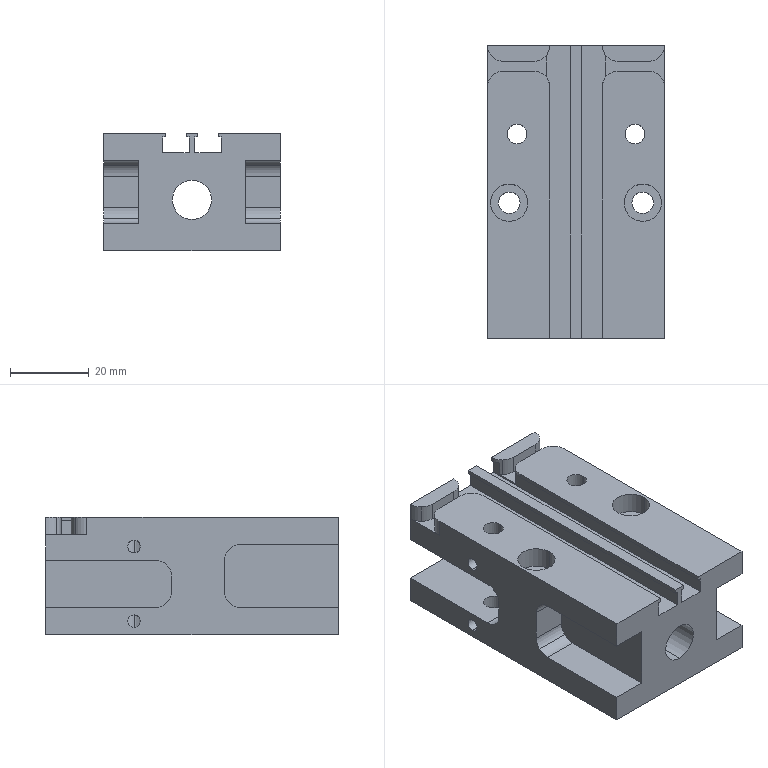Part | STEP file | PN_0068^seat_default | 1 solid | 116 faces | box 45 x 74.5 x 30 mm | volume 67519 mm3 | cylinder 62 | plane 50 | cone 4 | commonest cylinder face diameters 8 x32 3.24 x8 5 x8 2 x4 5.5 x4 9.5 x4